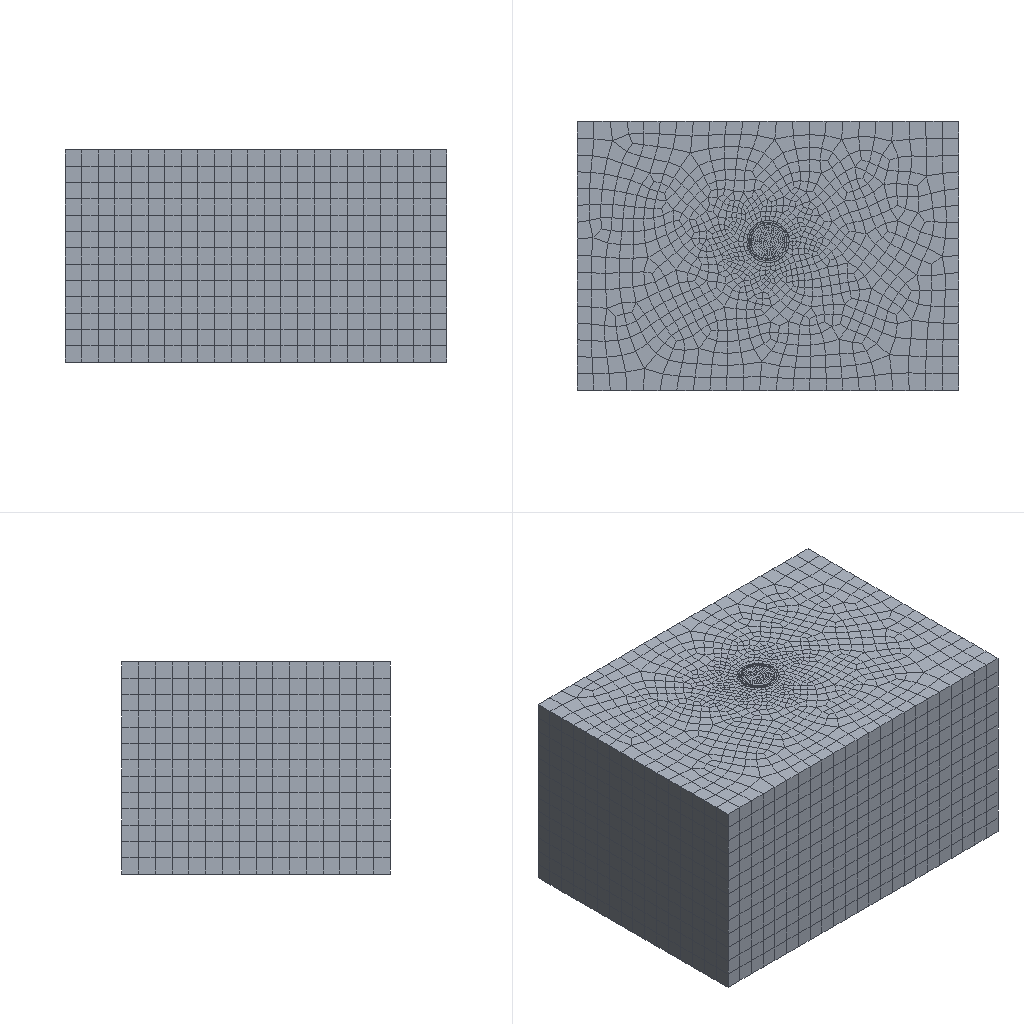Simulation study | abaqus
Set-up summary:
category,name,step,type,value,unit,region
solver,abaqus
solver,version,,,Abaqus/Standard 2020
units,not stated in the deck,,not stated
analysis,deck,,static,static
load_step,Step-1,Step-1,static
load_step,Step-2,Step-2,static
load_step,Step-3,Step-3,static
load_step,Step-4,Step-4,static
load_step,Step-5,Step-5,static
load_step,Step-6,Step-6,static
load_step,Step-7,Step-7,static
load_step,Step-8,Step-8,static
load_step,Step-9,Step-9,static
load_step,requested,,,9
mesh,nodes,,,42071
mesh,elements,,,36226
element_type,C3D8R,,solid,36226
load,load commands in deck,,count,9
bc,support commands in deck,,count,3
material,CHENQI,,in results
material,DOUGOU,,in results
material,SOIL,,in results
material,ZHUJIANG,,in results
check,setup vs results,,match,"per instance, exact: element labels, types and connectivity; labels of the nodes the elements use; coordinates of those nodes at SINGLE_PRECISION in 1 of 4 instance(s)"
Abaqus input file, long lists of numbers shortened:
*Heading
** Job name: Job-1 Model name: Model-1
** Generated by: Abaqus/CAE 2020
*Preprint, echo=NO, model=NO, history=NO, contact=NO
**
** PARTS
**
*Part, name=chenqi
*Node
      1,   1904.265,  -1460.744,           0.
      2,   2399.187,  -62.468,           0.
** (2198 more lines like these left out)
*Element, type=C3D8R
   1,   58,   86,   92,   72,    3,   31,   37,   17
   2,   73,   92,   86,   59,   18,   37,   31,    4
** (1324 more lines like these left out)
*Nset, nset=Set-1, generate
    1,  2200,     1
*Elset, elset=Set-1, generate
    1,  1326,     1
** Section: chenqi
*Solid Section, elset=Set-1, material=chenqi
,
*End Part
**
*Part, name=chip
*Node
      1,   678.8,  -2302.006,       12000.
      2,   678.8,  -2302.006,        9000.
** (23385 more lines like these left out)
*Element, type=C3D8R
   1,  613,   25,   26,  768, 6305, 1027, 1028, 6460
   2,  643,   68,   69,  644, 6335, 1070, 1071, 6336
** (20968 more lines like these left out)
*Nset, nset=Set-1
    17,    18,    19,    20,    21,    22,    23,    24,   489,   490,   491,   492,   493,   494,   495,   496
   497,   498,   499,   500,   501,   502,   503,   504,   505,   506,   507,   508,   509,   510,   511,   512
** (159 more lines like these left out)
*Elset, elset=Set-1, generate
 18874,  20970,      1
*Nset, nset=Set-2
    13,    14,    15,    16,    17,    18,    19,    20,   415,   416,   417,   418,   419,   420,   421,   422
   423,   424,   425,   426,   427,   428,   429,   430,   431,   432,   433,   434,   435,   436,   437,   438
** (159 more lines like these left out)
*Elset, elset=Set-2, generate
 16777,  18873,      1
*Nset, nset=Set-3
    10,    11,    12,    13,    14,    15,    16,   348,   349,   350,   351,   352,   353,   354,   355,   356
   357,   358,   359,   360,   361,   362,   363,   364,   365,   366,   367,   368,   369,   370,   371,   372
** (159 more lines like these left out)
*Elset, elset=Set-3, generate
 14680,  16776,      1
*Nset, nset=Set-4
     8,     9,    10,    11,    12,   288,   289,   290,   291,   292,   293,   294,   295,   296,   297,   298
   299,   300,   301,   302,   303,   304,   305,   306,   307,   308,   309,   310,   311,   312,   313,   314
** (159 more lines like these left out)
*Elset, elset=Set-4, generate
 12583,  14679,      1
*Nset, nset=Set-5
     6,     7,     8,     9,   228,   229,   230,   231,   232,   233,   234,   235,   236,   237,   238,   239
   240,   241,   242,   243,   244,   245,   246,   247,   248,   249,   250,   251,   252,   253,   254,   255
** (159 more lines like these left out)
*Elset, elset=Set-5, generate
 10486,  12582,      1
*Nset, nset=Set-6
     1,     6,     7,    25,    26,    27,    28,    29,    30,    31,    32,    33,    34,    35,    36,    37
    38,    39,    40,    41,    42,    43,    44,    45,    46,    47,    48,    49,    50,    51,    52,    53
** (159 more lines like these left out)
*Elset, elset=Set-6, generate
  8389,  10485,      1
*Nset, nset=Set-7
    1,    2,    3,   25,   26,   27,   28,   29,   30,   31,   32,   33,   34,   35,   36,   37
   38,   39,   40,   41,   42,   43,   44,   45,   46,   47,   48,   49,   50,   51,   52,   53
** (159 more lines like these left out)
*Elset, elset=Set-7, generate
    1,  2097,     1
*Nset, nset=Set-8
    2,    3,    4,   78,   79,   80,   81,   82,   83,   84,   85,   86,   87,   88,   89,   90
   91,   92,   93,   94,   95,   96,   97,   98,   99,  100,  101,  102,  103,  104,  105,  106
** (159 more lines like these left out)
*Elset, elset=Set-8, generate
 2098,  4194,     1
*Nset, nset=Set-9
     4,     5,   130,   131,   132,   133,   134,   135,   136,   137,   138,   139,   140,   141,   142,   143
   144,   145,   146,   147,   148,   149,   150,   151,   152,   153,   154,   155,   156,   157,   158,   159
** (304 more lines like these left out)
*Elset, elset=Set-9, generate
 4195,  8388,     1
*Nset, nset=duiying-1
     1,     2,     3,     4,     5,     6,     7,     8,     9,    10,    11,    12,    13,    14,    15,    16
    17,    18,    19,    20,    25,    26,    27,    28,    29,    30,    31,    32,    33,    34,    35,    36
** (1316 more lines like these left out)
*Elset, elset=duiying-1, generate
     1,  18873,      1
*Nset, nset=duiying-2
     1,     2,     3,     4,     5,     6,     7,     8,     9,    10,    11,    12,    13,    14,    15,    16
    25,    26,    27,    28,    29,    30,    31,    32,    33,    34,    35,    36,    37,    38,    39,    40
** (1171 more lines like these left out)
*Elset, elset=duiying-2, generate
     1,  16776,      1
*Nset, nset=duiying-3
     1,     2,     3,     4,     5,     6,     7,     8,     9,    10,    11,    12,    25,    26,    27,    28
    29,    30,    31,    32,    33,    34,    35,    36,    37,    38,    39,    40,    41,    42,    43,    44
** (1026 more lines like these left out)
*Elset, elset=duiying-3, generate
     1,  14679,      1
*Nset, nset=duiying-4
     1,     2,     3,     4,     5,     6,     7,     8,     9,    25,    26,    27,    28,    29,    30,    31
    32,    33,    34,    35,    36,    37,    38,    39,    40,    41,    42,    43,    44,    45,    46,    47
** (882 more lines like these left out)
*Elset, elset=duiying-4, generate
     1,  12582,      1
*Nset, nset=duiying-5
     1,     2,     3,     4,     5,     6,     7,    25,    26,    27,    28,    29,    30,    31,    32,    33
    34,    35,    36,    37,    38,    39,    40,    41,    42,    43,    44,    45,    46,    47,    48,    49
** (737 more lines like these left out)
*Elset, elset=duiying-5, generate
     1,  10485,      1
*Nset, nset=duiyng-6
     1,     2,     3,     4,     5,    25,    26,    27,    28,    29,    30,    31,    32,    33,    34,    35
    36,    37,    38,    39,    40,    41,    42,    43,    44,    45,    46,    47,    48,    49,    50,    51
** (593 more lines like these left out)
*Elset, elset=duiyng-6, generate
    1,  8388,     1
*Nset, nset=duiyng-7
     2,     3,     4,     5,    78,    79,    80,    81,    82,    83,    84,    85,    86,    87,    88,    89
    90,    91,    92,    93,    94,    95,    96,    97,    98,    99,   100,   101,   102,   103,   104,   105
** (448 more lines like these left out)
*Elset, elset=duiyng-7, generate
 2098,  8388,     1
*Nset, nset=duiying-8
     4,     5,   130,   131,   132,   133,   134,   135,   136,   137,   138,   139,   140,   141,   142,   143
   144,   145,   146,   147,   148,   149,   150,   151,   152,   153,   154,   155,   156,   157,   158,   159
** (304 more lines like these left out)
*Elset, elset=duiying-8, generate
 4195,  8388,     1
*Nset, nset=Set-19, generate
     1,  23387,      1
*Elset, elset=Set-19, generate
     1,  20970,      1
** Section: chip
*Solid Section, elset=Set-19, material=soil
,
*End Part
**
*Part, name=soil
*Node
      1,    29614.959,  -18470.371,           0.
      2,    29997.334,  -16873.537,           0.
** (14502 more lines like these left out)
*Element, type=C3D8R
    1,   113,    12,    38,   145,  1149,  1048,  1074,  1181
    2,   239,   198,   173,   199,  1275,  1234,  1209,  1235
** (12738 more lines like these left out)
*Nset, nset=Set-1, generate
     1,  14504,      1
*Elset, elset=Set-1, generate
     1,  12740,      1
** Section: soil
*Solid Section, elset=Set-1, material=soil
,
*End Part
**
*Part, name=zhujiang
*Node
      1,   2405.718,  -1225.774,           0.
      2,   2666.759,   422.373,           0.
** (1978 more lines like these left out)
*Element, type=C3D8R
   1,   93,  100,  101,   75,   38,   45,   46,   20
   2,   88,  102,  101,   59,   33,   47,   46,    4
** (1188 more lines like these left out)
*Nset, nset=Set-1, generate
    1,  1980,     1
*Elset, elset=Set-1, generate
    1,  1190,     1
** Section: zhujiang
*Solid Section, elset=Set-1, material=zhujiang
,
*End Part
**
**
** ASSEMBLY
**
*Assembly, name=Assembly
**
*Instance, name=soil-1, part=soil
*End Instance
**
*Instance, name=chenqi-1, part=chenqi
      27000.,      -17000.,           0.
*End Instance
**
*Instance, name=zhujiang-1, part=zhujiang
      27000.,      -17000.,           0.
*End Instance
**
*Instance, name=chip-1, part=chip
      27000.,      -17000.,           0.
*End Instance
**
*Nset, nset=Set-1, instance=soil-1
    15,    16,    76,    77,    78,    79,    80,    81,    82,    83,    84,    85,    86,    87,    88,    89
    90,    91,    92,    93,    94,    95,    96,    97,  1051,  1052,  1112,  1113,  1114,  1115,  1116,  1117
** (19 more lines like these left out)
*Elset, elset=Set-1, instance=soil-1
    48,    49,    61,    92,   709,   738,   739,   740,   742,   773,   789,   797,   804,   819,   830,   841
   844,   858,   863,   864,   867,   870,   874,  1028,  1029,  1041,  1072,  1689,  1718,  1719,  1720,  1722
** (17 more lines like these left out)
*Nset, nset=Set-2, instance=soil-1
    13,    14,    15,    16,    61,    62,    63,    64,    65,    66,    67,    68,    69,    70,    71,    72
    73,    74,    75,    98,    99,   100,   101,   102,   103,   104,   105,   106,   107,   108,   109,   110
** (28 more lines like these left out)
*Elset, elset=Set-2, instance=soil-1
    32,    48,    60,    61,    79,    91,   677,   764,   814,   817,   824,   825,   833,   835,   836,   840
   843,   848,   859,   862,   865,   872,   873,   875,   877,   880,   881,   882,   884,   885,   886,   891
** (24 more lines like these left out)
*Nset, nset=Set-3, instance=chip-1
    13,    14,    15,    16,    17,    18,    19,    20,    21,    22,    23,    24,   415,   416,   417,   418
   419,   420,   421,   422,   423,   424,   425,   426,   427,   428,   429,   430,   431,   432,   433,   434
** (304 more lines like these left out)
*Elset, elset=Set-3, instance=chip-1, generate
 16777,  20970,      1
*Nset, nset=Set-4, instance=chip-1
    10,    11,    12,    13,    14,    15,    16,    17,    18,    19,    20,    21,    22,    23,    24,   348
   349,   350,   351,   352,   353,   354,   355,   356,   357,   358,   359,   360,   361,   362,   363,   364
** (448 more lines like these left out)
*Elset, elset=Set-4, instance=chip-1, generate
 14680,  20970,      1
*Nset, nset=Set-5, instance=chip-1
     8,     9,    10,    11,    12,    13,    14,    15,    16,    17,    18,    19,    20,    21,    22,    23
    24,   288,   289,   290,   291,   292,   293,   294,   295,   296,   297,   298,   299,   300,   301,   302
** (593 more lines like these left out)
*Elset, elset=Set-5, instance=chip-1, generate
 12583,  20970,      1
*Nset, nset=Set-6, instance=chip-1
     6,     7,     8,     9,    10,    11,    12,    13,    14,    15,    16,    17,    18,    19,    20,    21
    22,    23,    24,   228,   229,   230,   231,   232,   233,   234,   235,   236,   237,   238,   239,   240
** (737 more lines like these left out)
*Elset, elset=Set-6, instance=chip-1, generate
 10486,  20970,      1
*Nset, nset=Set-7, instance=chip-1
     1,     6,     7,     8,     9,    10,    11,    12,    13,    14,    15,    16,    17,    18,    19,    20
    21,    22,    23,    24,    25,    26,    27,    28,    29,    30,    31,    32,    33,    34,    35,    36
** (882 more lines like these left out)
*Elset, elset=Set-7, instance=chip-1, generate
  8389,  20970,      1
*Nset, nset=Set-8, instance=chip-1
     1,     2,     3,     6,     7,     8,     9,    10,    11,    12,    13,    14,    15,    16,    17,    18
    19,    20,    21,    22,    23,    24,    25,    26,    27,    28,    29,    30,    31,    32,    33,    34
** (1026 more lines like these left out)
*Elset, elset=Set-8, instance=chip-1
     1,     2,     3,     4,     5,     6,     7,     8,     9,    10,    11,    12,    13,    14,    15,    16
    17,    18,    19,    20,    21,    22,    23,    24,    25,    26,    27,    28,    29,    30,    31,    32
** (916 more lines like these left out)
*Nset, nset=Set-9, instance=chip-1
     1,     2,     3,     4,     6,     7,     8,     9,    10,    11,    12,    13,    14,    15,    16,    17
    18,    19,    20,    21,    22,    23,    24,    25,    26,    27,    28,    29,    30,    31,    32,    33
** (1171 more lines like these left out)
*Elset, elset=Set-9, instance=chip-1
     1,     2,     3,     4,     5,     6,     7,     8,     9,    10,    11,    12,    13,    14,    15,    16
    17,    18,    19,    20,    21,    22,    23,    24,    25,    26,    27,    28,    29,    30,    31,    32
** (1047 more lines like these left out)
*Nset, nset=Set-10, instance=chip-1, generate
     1,  23387,      1
*Elset, elset=Set-10, instance=chip-1, generate
     1,  20970,      1
*Nset, nset=Set-11, instance=soil-1
     1,     2,     3,     4,     5,     6,     7,     8,     9,    10,    11,    12,    13,    14,    15,    16
    17,    18,    19,    20,    21,    22,    23,    24,    25,    26,    27,    28,    29,    30,    31,    32
** (128 more lines like these left out)
*Elset, elset=Set-11, instance=soil-1
     1,     2,     3,     4,     5,     6,     7,     8,     9,    10,    11,    12,    13,    14,    15,    16
    17,    18,    19,    20,    21,    22,    23,    24,    25,    26,    27,    28,    29,    30,    31,    32
** (121 more lines like these left out)
*Elset, elset=_Surf-1_S2, internal, instance=chip-1, generate
 20738,  20970,      1
*Surface, type=ELEMENT, name=Surf-1
_Surf-1_S2, S2
*Elset, elset=_Surf-2_S2, internal, instance=chip-1, generate
 18641,  18873,      1
*Surface, type=ELEMENT, name=Surf-2
_Surf-2_S2, S2
*Elset, elset=_Surf-3_S2, internal, instance=chip-1, generate
 16544,  16776,      1
*Surface, type=ELEMENT, name=Surf-3
_Surf-3_S2, S2
*Elset, elset=_Surf-4_S1, internal, instance=chip-1, generate
 14680,  14912,      1
*Surface, type=ELEMENT, name=Surf-4
_Surf-4_S1, S1
*Elset, elset=_Surf-5_S2, internal, instance=chip-1, generate
 12350,  12582,      1
*Surface, type=ELEMENT, name=Surf-5
_Surf-5_S2, S2
*Elset, elset=_Surf-6_S2, internal, instance=chip-1, generate
 10253,  10485,      1
*Surface, type=ELEMENT, name=Surf-6
_Surf-6_S2, S2
*Elset, elset=_Surf-7_S1, internal, instance=chip-1, generate
 8389,  8621,     1
*Surface, type=ELEMENT, name=Surf-7
_Surf-7_S1, S1
*Elset, elset=_Surf-8_S1, internal, instance=chip-1, generate
   1,  233,    1
*Surface, type=ELEMENT, name=Surf-8
_Surf-8_S1, S1
*Elset, elset=_Surf-9_S1, internal, instance=chip-1, generate
 2098,  2330,     1
*Surface, type=ELEMENT, name=Surf-9
_Surf-9_S1, S1
*Elset, elset=_Surf-10_S1, internal, instance=chip-1, generate
 4195,  4427,     1
*Surface, type=ELEMENT, name=Surf-10
_Surf-10_S1, S1
*Elset, elset=_Surf-11_S2, internal, instance=chip-1, generate
 14447,  14679,      1
*Surface, type=ELEMENT, name=Surf-11
_Surf-11_S2, S2
*Elset, elset=_m_Surf-12_S4, internal, instance=chip-1
    1,    2,    3,    4,    5,    6,    7,    9,   10,   18,   19,   20,   37,   40,   42,   44
   45,   48,   49,   50,   58,   66,   71,   79,  211,  234,  235,  236,  237,  238,  239,  240
** (55 more lines like these left out)
*Elset, elset=_m_Surf-12_S6, internal, instance=chip-1
    11,    14,    15,    16,    22,    23,    24,    26,    29,    30,    32,    34,    36,    38,    39,    41
    43,    46,    54,   244,   247,   248,   249,   255,   256,   257,   259,   262,   263,   265,   267,   269
** (48 more lines like these left out)
*Elset, elset=_m_Surf-12_S3, internal, instance=chip-1
    13,    47,   246,   280,   479,   513,   712,   746,   945,   979,  1178,  1212,  1411,  1445,  1644,  1678
  1877,  1911,  2110,  2144,  2343,  2377,  2576,  2610,  2809,  2843,  3042,  3076,  3275,  3309,  3508,  3542
** (67 more lines like these left out)
*Elset, elset=_m_Surf-12_S5, internal, instance=chip-1
  8389,  8390,  8391,  8392,  8393,  8394,  8395,  8397,  8398,  8406,  8407,  8408,  8425,  8428,  8430,  8432
  8433,  8436,  8437,  8438,  8446,  8454,  8459,  8467,  8599,  8622,  8623,  8624,  8625,  8626,  8627,  8628
** (83 more lines like these left out)
*Elset, elset=_m_Surf-12_S2, internal, instance=chip-1, generate
 8156,  8388,     1
*Surface, type=ELEMENT, name=m_Surf-12
_m_Surf-12_S4, S4
_m_Surf-12_S6, S6
_m_Surf-12_S2, S2
_m_Surf-12_S3, S3
_m_Surf-12_S5, S5
*Elset, elset=_m_Surf-14_S5, internal, instance=chenqi-1
    1,    4,    7,   14,   30,   35,   38,   41,   48,   64,   69,   72,   75,   82,   98,  103
  106,  109,  116,  132,  137,  140,  143,  150,  166,  171,  174,  177,  184,  200,  205,  208
** (11 more lines like these left out)
*Elset, elset=_m_Surf-14_S3, internal, instance=chenqi-1
    2,    3,   16,   24,   25,   28,   36,   37,   50,   58,   59,   62,   70,   71,   84,   92
   93,   96,  104,  105,  118,  126,  127,  130,  138,  139,  152,  160,  161,  164,  172,  173
** (13 more lines like these left out)
*Elset, elset=_m_Surf-14_S4, internal, instance=chenqi-1
    9,   19,   20,   31,   43,   53,   54,   65,   77,   87,   88,   99,  111,  121,  122,  133
  145,  155,  156,  167,  179,  189,  190,  201,  213,  223,  224,  235,  247,  257,  258,  269
** (8 more lines like these left out)
*Elset, elset=_m_Surf-14_S6, internal, instance=chenqi-1
   11,   12,   13,   15,   22,   26,   34,   45,   46,   47,   49,   56,   60,   68,   79,   80
   81,   83,   90,   94,  102,  113,  114,  115,  117,  124,  128,  136,  147,  148,  149,  151
** (16 more lines like these left out)
*Surface, type=ELEMENT, name=m_Surf-14
_m_Surf-14_S5, S5
_m_Surf-14_S3, S3
_m_Surf-14_S4, S4
_m_Surf-14_S6, S6
*Elset, elset=_m_Surf-16_S6, internal, instance=zhujiang-1
    1,    4,    9,   10,   18,   20,   25,   27,   32,   34,   35,   38,   43,   44,   52,   54
   59,   61,   66,   68,   69,   72,   77,   78,   86,   88,   93,   95,  100,  102,  103,  106
** (20 more lines like these left out)
*Elset, elset=_m_Surf-16_S3, internal, instance=zhujiang-1
    3,    7,   15,   21,   22,   37,   41,   49,   55,   56,   71,   75,   83,   89,   90,  105
  109,  117,  123,  124,  139,  143,  151,  157,  158,  173,  177,  185,  191,  192,  207,  211
** (9 more lines like these left out)
*Elset, elset=_m_Surf-16_S4, internal, instance=zhujiang-1
   11,   17,   31,   45,   51,   65,   79,   85,   99,  113,  119,  133,  147,  153,  167,  181
  187,  201,  215,  221,  235,  249,  255,  269,  283,  289,  303,  317,  323,  337,  351,  357
** (5 more lines like these left out)
*Elset, elset=_m_Surf-16_S5, internal, instance=zhujiang-1
   12,   13,   14,   29,   46,   47,   48,   63,   80,   81,   82,   97,  114,  115,  116,  131
  148,  149,  150,  165,  182,  183,  184,  199,  216,  217,  218,  233,  250,  251,  252,  267
** (7 more lines like these left out)
*Surface, type=ELEMENT, name=m_Surf-16
_m_Surf-16_S6, S6
_m_Surf-16_S3, S3
_m_Surf-16_S4, S4
_m_Surf-16_S5, S5
*Elset, elset=_s_Surf-12_S3, internal, instance=chenqi-1
    1,   14,   27,   35,   48,   61,   69,   82,   95,  103,  116,  129,  137,  150,  163,  171
  184,  197,  205,  218,  231,  239,  252,  265,  273,  286,  299,  307,  320,  333,  341,  354
** (6 more lines like these left out)
*Elset, elset=_s_Surf-12_S5, internal, instance=chenqi-1
    2,    3,    8,   10,   36,   37,   42,   44,   70,   71,   76,   78,  104,  105,  110,  112
  138,  139,  144,  146,  172,  173,  178,  180,  206,  207,  212,  214,  240,  241,  246,  248
** (8 more lines like these left out)
*Elset, elset=_s_Surf-12_S6, internal, instance=chenqi-1
    5,   18,   21,   33,   39,   52,   55,   67,   73,   86,   89,  101,  107,  120,  123,  135
  141,  154,  157,  169,  175,  188,  191,  203,  209,  222,  225,  237,  243,  256,  259,  271
** (8 more lines like these left out)
*Elset, elset=_s_Surf-12_S4, internal, instance=chenqi-1
    6,   11,   12,   13,   17,   22,   23,   29,   32,   40,   45,   46,   47,   51,   56,   57
   63,   66,   74,   79,   80,   81,   85,   90,   91,   97,  100,  108,  113,  114,  115,  119
** (20 more lines like these left out)
*Surface, type=ELEMENT, name=s_Surf-12
_s_Surf-12_S3, S3
_s_Surf-12_S5, S5
_s_Surf-12_S6, S6
_s_Surf-12_S4, S4
*Elset, elset=_s_Surf-14_S6, internal, instance=zhujiang-1
    2,    5,    6,   11,   17,   36,   39,   40,   45,   51,   70,   73,   74,   79,   85,  104
  107,  108,  113,  119,  138,  141,  142,  147,  153,  172,  175,  176,  181,  187,  206,  209
** (9 more lines like these left out)
*Elset, elset=_s_Surf-14_S3, internal, instance=zhujiang-1
    8,   12,   13,   14,   24,   26,   28,   30,   42,   46,   47,   48,   58,   60,   62,   64
   76,   80,   81,   82,   92,   94,   96,   98,  110,  114,  115,  116,  126,  128,  130,  132
** (16 more lines like these left out)
*Elset, elset=_s_Surf-14_S4, internal, instance=zhujiang-1
    9,   10,   16,   23,   33,   43,   44,   50,   57,   67,   77,   78,   84,   91,  101,  111
  112,  118,  125,  135,  145,  146,  152,  159,  169,  179,  180,  186,  193,  203,  213,  214
** (9 more lines like these left out)
*Elset, elset=_s_Surf-14_S5, internal, instance=zhujiang-1
   19,   22,   53,   56,   87,   90,  121,  124,  155,  158,  189,  192,  223,  226,  257,  260
  291,  294,  325,  328,  359,  362,  393,  396,  427,  430,  461,  464,  495,  498,  529,  532
** (3 more lines like these left out)
*Surface, type=ELEMENT, name=s_Surf-14
_s_Surf-14_S6, S6
_s_Surf-14_S3, S3
_s_Surf-14_S4, S4
_s_Surf-14_S5, S5
*Elset, elset=_s_Surf-16_S4, internal, instance=soil-1
     1,     5,    10,    16,    20,    23,    25,    26,    29,    30,    93,    94,    96,    97,    98,   101
   103,   104,   981,   985,   990,   996,  1000,  1003,  1005,  1006,  1009,  1010,  1073,  1074,  1076,  1077
** (13 more lines like these left out)
*Elset, elset=_s_Surf-16_S6, internal, instance=soil-1
     3,     8,     9,    11,    27,    39,    67,    70,    74,    85,    87,   106,   983,   988,   989,   991
  1007,  1019,  1047,  1050,  1054,  1065,  1067,  1086,  1963,  1968,  1969,  1971,  1987,  1999,  2027,  2030
** (8 more lines like these left out)
*Elset, elset=_s_Surf-16_S3, internal, instance=soil-1
    12,    18,   992,   998,  1972,  1978,  2952,  2958,  3932,  3938,  4912,  4918,  5892,  5898,  6872,  6878
  7852,  7858,  8832,  8838,  9812,  9818, 10792, 10798, 11772, 11778
*Elset, elset=_s_Surf-16_S5, internal, instance=soil-1
    15,    95,   995,  1075,  1975,  2055,  2955,  3035,  3935,  4015,  4915,  4995,  5895,  5975,  6875,  6955
  7855,  7935,  8835,  8915,  9815,  9895, 10795, 10875, 11775, 11855
*Surface, type=ELEMENT, name=s_Surf-16
_s_Surf-16_S4, S4
_s_Surf-16_S6, S6
_s_Surf-16_S3, S3
_s_Surf-16_S5, S5
** Constraint: Constraint-1
*Tie, name=Constraint-1, adjust=yes
s_Surf-12, m_Surf-12
** Constraint: Constraint-2
*Tie, name=Constraint-2, adjust=yes
s_Surf-14, m_Surf-14
** Constraint: Constraint-3
*Tie, name=Constraint-3, adjust=yes
s_Surf-16, m_Surf-16
*End Assembly
**
** MATERIALS
**
*Material, name=chenqi
*Density
 2.5e-09,
*Elastic
30000., 0.25
*Material, name=dougou
*Density
 7.5e-09,
*Elastic
210000., 0.2
*Material, name=soil
*Density
 2e-09,
*Elastic
8., 0.27
*Mohr Coulomb
29.,16.
*Mohr Coulomb Hardening
15.,0.
*Material, name=zhujiang
*Density
 2.4e-09,
*Elastic
 1.5, 0.2
**
** BOUNDARY CONDITIONS
**
** Name: BC-3 Type: 位移/转角
*Boundary
Set-11, 3, 3
** ----------------------------------------------------------------
**
** STEP: Step-1
**
*Step, name=Step-1, nlgeom=NO
*Static
0.001, 1., 1e-05, 1.
**
** BOUNDARY CONDITIONS
**
** Name: BC-1 Type: 对称/反对称/完全固定
*Boundary
Set-1, ENCASTRE
** Name: BC-2 Type: 位移/转角
*Boundary
Set-2, 1, 1
**
** LOADS
**
** Name: Load-1   Type: Pressure
*Dsload
Surf-1, P, 0.1
** Name: Load-2   Type: Pressure
*Dsload
Surf-2, P, 0.1
** Name: Load-3   Type: Pressure
*Dsload
Surf-3, P, 0.1
** Name: Load-4   Type: Pressure
*Dsload
Surf-11, P, 0.1
** Name: Load-5   Type: Pressure
*Dsload
Surf-5, P, 0.1
** Name: Load-6   Type: Pressure
*Dsload
Surf-6, P, 0.1
** Name: Load-7   Type: Pressure
*Dsload
Surf-8, P, 0.1
** Name: Load-8   Type: Pressure
*Dsload
Surf-9, P, 0.1
** Name: Load-9   Type: Pressure
*Dsload
Surf-10, P, 0.1
**
** INTERACTIONS
**
** Interaction: Int-1
*Model Change, remove
chip-1.Set-1,
**
** OUTPUT REQUESTS
**
*Restart, write, frequency=0
**
** FIELD OUTPUT: F-Output-1
**
*Output, field
*Node Output
CF, RF, U
*Element Output, directions=YES
E, LE, MISES, PE, PEEQ, PEMAG, S, STATUS
*Contact Output
CDISP, CSTRESS
**
** HISTORY OUTPUT: H-Output-1
**
*Output, history, variable=PRESELECT
*End Step
** ----------------------------------------------------------------
**
** STEP: Step-2
**
*Step, name=Step-2, nlgeom=NO
*Static
1., 1., 1e-05, 1.
**
** INTERACTIONS
**
** Interaction: Int-2
*Model Change, remove
Set-3,
**
** OUTPUT REQUESTS
**
*Restart, write, frequency=0
**
** FIELD OUTPUT: F-Output-1
**
*Output, field
*Node Output
CF, RF, U
*Element Output, directions=YES
E, LE, MISES, PE, PEEQ, PEMAG, S, STATUS
*Contact Output
CDISP, CSTRESS
**
** HISTORY OUTPUT: H-Output-1
**
*Output, history, variable=PRESELECT
*End Step
** ----------------------------------------------------------------
**
** STEP: Step-3
**
*Step, name=Step-3, nlgeom=NO
*Static
1., 1., 1e-05, 1.
**
** INTERACTIONS
**
** Interaction: Int-3
*Model Change, remove
Set-4,
**
** OUTPUT REQUESTS
**
*Restart, write, frequency=0
**
** FIELD OUTPUT: F-Output-1
**
*Output, field
*Node Output
CF, RF, U
*Element Output, directions=YES
E, LE, MISES, PE, PEEQ, PEMAG, S, STATUS
*Contact Output
CDISP, CSTRESS
**
** HISTORY OUTPUT: H-Output-1
**
*Output, history, variable=PRESELECT
*End Step
** ----------------------------------------------------------------
**
** STEP: Step-4
**
*Step, name=Step-4, nlgeom=NO
*Static
1., 1., 1e-05, 1.
**
** INTERACTIONS
**
** Interaction: Int-4
*Model Change, remove
Set-5,
**
** OUTPUT REQUESTS
**
*Restart, write, frequency=0
**
** FIELD OUTPUT: F-Output-1
**
*Output, field
*Node Output
CF, RF, U
*Element Output, directions=YES
E, LE, MISES, PE, PEEQ, PEMAG, S, STATUS
*Contact Output
CDISP, CSTRESS
**
** HISTORY OUTPUT: H-Output-1
**
*Output, history, variable=PRESELECT
*End Step
** ----------------------------------------------------------------
**
** STEP: Step-5
**
*Step, name=Step-5, nlgeom=NO
*Static
1., 1., 1e-05, 1.
**
** INTERACTIONS
**
** Interaction: Int-5
*Model Change, remove
Set-6,
**
** OUTPUT REQUESTS
**
*Restart, write, frequency=0
**
** FIELD OUTPUT: F-Output-1
**
*Output, field
*Node Output
CF, RF, U
*Element Output, directions=YES
E, LE, MISES, PE, PEEQ, PEMAG, S, STATUS
*Contact Output
CDISP, CSTRESS
**
** HISTORY OUTPUT: H-Output-1
**
*Output, history, variable=PRESELECT
*End Step
** ----------------------------------------------------------------
**
** STEP: Step-6
**
*Step, name=Step-6, nlgeom=NO
*Static
1., 1., 1e-05, 1.
**
** INTERACTIONS
**
** Interaction: Int-6
*Model Change, remove
Set-7,
**
** OUTPUT REQUESTS
**
*Restart, write, frequency=0
**
** FIELD OUTPUT: F-Output-1
**
*Output, field
*Node Output
CF, RF, U
*Element Output, directions=YES
E, LE, MISES, PE, PEEQ, PEMAG, S, STATUS
*Contact Output
CDISP, CSTRESS
**
** HISTORY OUTPUT: H-Output-1
**
*Output, history, variable=PRESELECT
*End Step
** ----------------------------------------------------------------
**
** STEP: Step-7
**
*Step, name=Step-7, nlgeom=NO
*Static
1., 1., 1e-05, 1.
**
** INTERACTIONS
**
** Interaction: Int-7
*Model Change, remove
Set-8,
**
** OUTPUT REQUESTS
**
*Restart, write, frequency=0
**
** FIELD OUTPUT: F-Output-1
**
*Output, field
*Node Output
CF, RF, U
*Element Output, directions=YES
E, LE, MISES, PE, PEEQ, PEMAG, S, STATUS
*Contact Output
CDISP, CSTRESS
**
** HISTORY OUTPUT: H-Output-1
**
*Output, history, variable=PRESELECT
*End Step
** ----------------------------------------------------------------
**
** STEP: Step-8
**
*Step, name=Step-8, nlgeom=NO
*Static
1., 1., 1e-05, 1.
**
** INTERACTIONS
**
** Interaction: Int-8
*Model Change, remove
Set-9,
**
** OUTPUT REQUESTS
**
*Restart, write, frequency=0
**
** FIELD OUTPUT: F-Output-1
**
*Output, field
*Node Output
CF, RF, U
*Element Output, directions=YES
E, LE, MISES, PE, PEEQ, PEMAG, S, STATUS
*Contact Output
CDISP, CSTRESS
**
** HISTORY OUTPUT: H-Output-1
**
*Output, history, variable=PRESELECT
*End Step
** ----------------------------------------------------------------
**
** STEP: Step-9
**
*Step, name=Step-9, nlgeom=NO
*Static
1., 1., 1e-05, 1.
**
** INTERACTIONS
**
** Interaction: Int-9
*Model Change, remove
Set-10,
**
** OUTPUT REQUESTS
**
*Restart, write, frequency=0
**
** FIELD OUTPUT: F-Output-1
**
*Output, field
*Node Output
CF, RF, U
*Element Output, directions=YES
E, LE, MISES, PE, PEEQ, PEMAG, S, STATUS
*Contact Output
CDISP, CSTRESS
**
** HISTORY OUTPUT: H-Output-1
**
*Output, history, variable=PRESELECT
*End Step
Results summary:
result,step,,completed,increments=17 time=1.0/1.0
result,step,,completed,increments=1 time=1.0/1.0
result,step,,completed,increments=1 time=1.0/1.0
result,step,,completed,increments=1 time=1.0/1.0
result,step,,completed,increments=1 time=1.0/1.0
result,step,,completed,increments=1 time=1.0/1.0
result,step,,completed,increments=1 time=1.0/1.0
result,step,,completed,increments=1 time=1.0/1.0
result,step,,completed,increments=1 time=1.0/1.0
result,analysis,,,static
result,last_loadstep,,,9
result,primary field,,,U
result,reaction total,,FX,0.000223,model units
result,reaction total,,FY,0.000242,model units
result,reaction total,,FZ,-0.000137,model units